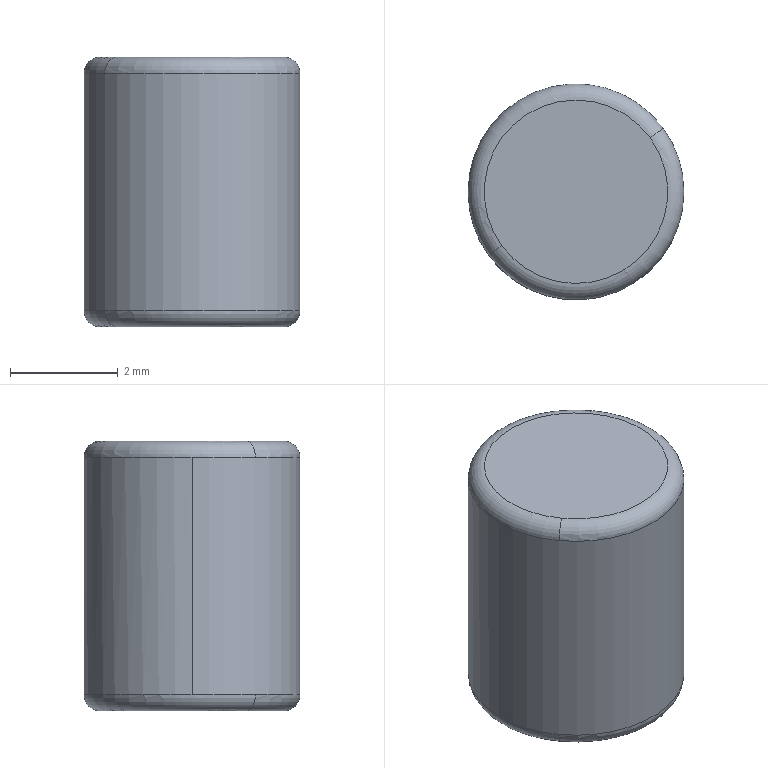Part | 1 solid | 8 faces | box 4 x 4 x 5 mm | volume 62.363 mm3 | torus 4 | cylinder 2 | plane 2 | commonest cylinder face diameters 4 x2
STEP:
#1=CARTESIAN_POINT('',(0.,0.,0.));
#2=DIRECTION('',(0.,0.,1.));
#3=DIRECTION('',(1.,0.,0.));
#4=AXIS2_PLACEMENT_3D('',#1,#2,#3);
#5=CARTESIAN_POINT('',(-242.098,492.5,-190.901));
#6=VERTEX_POINT('',#5);
#7=CARTESIAN_POINT('',(-242.098,492.5,-195.301));
#8=VERTEX_POINT('',#7);
#9=CARTESIAN_POINT('',(-242.098,492.5,-190.901));
#10=DIRECTION('',(0.,0.,-1.));
#11=VECTOR('',#10,1.);
#12=LINE('',#9,#11);
#13=CARTESIAN_POINT('',(-240.098,492.5,-190.601));
#14=DIRECTION('',(0.,0.,-1.));
#15=DIRECTION('',(0.,-1.,0.));
#16=AXIS2_PLACEMENT_3D('',#13,#14,#15);
#17=CYLINDRICAL_SURFACE('',#16,2.);
#18=CARTESIAN_POINT('',(1.571,0.3));
#19=DIRECTION('',(0.,1.));
#20=VECTOR('',#19,1.);
#21=LINE('',#18,#20);
#22=(GEOMETRIC_REPRESENTATION_CONTEXT(2)PARAMETRIC_REPRESENTATION_CONTEXT()REPRESENTATION_CONTEXT('',''));
#23=DEFINITIONAL_REPRESENTATION('',(#21),#22);
#24=PCURVE('',#17,#23);
#25=CARTESIAN_POINT('',(-240.098,492.5,-190.601));
#26=DIRECTION('',(0.,0.,-1.));
#27=DIRECTION('',(0.,1.,0.));
#28=AXIS2_PLACEMENT_3D('',#25,#26,#27);
#29=CYLINDRICAL_SURFACE('',#28,2.);
#30=CARTESIAN_POINT('',(4.712,0.3));
#31=DIRECTION('',(0.,1.));
#32=VECTOR('',#31,1.);
#33=LINE('',#30,#32);
#34=(GEOMETRIC_REPRESENTATION_CONTEXT(2)PARAMETRIC_REPRESENTATION_CONTEXT()REPRESENTATION_CONTEXT('',''));
#35=DEFINITIONAL_REPRESENTATION('',(#33),#34);
#36=PCURVE('',#29,#35);
#37=SURFACE_CURVE('',#12,(#24,#36),.PCURVE_S1.);
#38=EDGE_CURVE('',#6,#8,#37,.T.);
#39=ORIENTED_EDGE('',*,*,#38,.F.);
#40=CARTESIAN_POINT('',(-238.48,493.676,-190.901));
#41=VERTEX_POINT('',#40);
#42=CARTESIAN_POINT('',(-240.098,492.5,-190.901));
#43=DIRECTION('',(0.,0.,-1.));
#44=DIRECTION('',(-1.,0.,0.));
#45=AXIS2_PLACEMENT_3D('',#42,#43,#44);
#46=CIRCLE('',#45,2.);
#47=CARTESIAN_POINT('',(1.571,0.3));
#48=DIRECTION('',(1.,0.));
#49=VECTOR('',#48,1.);
#50=LINE('',#47,#49);
#51=(GEOMETRIC_REPRESENTATION_CONTEXT(2)PARAMETRIC_REPRESENTATION_CONTEXT()REPRESENTATION_CONTEXT('',''));
#52=DEFINITIONAL_REPRESENTATION('',(#50),#51);
#53=PCURVE('',#17,#52);
#54=CARTESIAN_POINT('',(-240.098,492.5,-190.901));
#55=DIRECTION('',(0.,0.,-1.));
#56=DIRECTION('',(0.5878,-0.809,0.));
#57=AXIS2_PLACEMENT_3D('',#54,#55,#56);
#58=TOROIDAL_SURFACE('',#57,1.7,0.3);
#59=CARTESIAN_POINT('',(2.199,6.283));
#60=DIRECTION('',(1.,0.));
#61=VECTOR('',#60,1.);
#62=LINE('',#59,#61);
#63=(GEOMETRIC_REPRESENTATION_CONTEXT(2)PARAMETRIC_REPRESENTATION_CONTEXT()REPRESENTATION_CONTEXT('',''));
#64=DEFINITIONAL_REPRESENTATION('',(#62),#63);
#65=PCURVE('',#58,#64);
#66=SURFACE_CURVE('',#46,(#53,#65),.PCURVE_S1.);
#67=EDGE_CURVE('',#6,#41,#66,.T.);
#68=ORIENTED_EDGE('',*,*,#67,.T.);
#69=CARTESIAN_POINT('',(-238.098,492.5,-190.901));
#70=VERTEX_POINT('',#69);
#71=CARTESIAN_POINT('',(-240.098,492.5,-190.901));
#72=DIRECTION('',(0.,0.,-1.));
#73=DIRECTION('',(-1.,0.,0.));
#74=AXIS2_PLACEMENT_3D('',#71,#72,#73);
#75=CIRCLE('',#74,2.);
#76=CARTESIAN_POINT('',(1.571,0.3));
#77=DIRECTION('',(1.,0.));
#78=VECTOR('',#77,1.);
#79=LINE('',#76,#78);
#80=(GEOMETRIC_REPRESENTATION_CONTEXT(2)PARAMETRIC_REPRESENTATION_CONTEXT()REPRESENTATION_CONTEXT('',''));
#81=DEFINITIONAL_REPRESENTATION('',(#79),#80);
#82=PCURVE('',#17,#81);
#83=CARTESIAN_POINT('',(-240.098,492.5,-190.901));
#84=DIRECTION('',(0.,0.,-1.));
#85=DIRECTION('',(-0.5878,0.809,0.));
#86=AXIS2_PLACEMENT_3D('',#83,#84,#85);
#87=TOROIDAL_SURFACE('',#86,1.7,0.3);
#88=CARTESIAN_POINT('',(-0.9425,6.283));
#89=DIRECTION('',(1.,0.));
#90=VECTOR('',#89,1.);
#91=LINE('',#88,#90);
#92=(GEOMETRIC_REPRESENTATION_CONTEXT(2)PARAMETRIC_REPRESENTATION_CONTEXT()REPRESENTATION_CONTEXT('',''));
#93=DEFINITIONAL_REPRESENTATION('',(#91),#92);
#94=PCURVE('',#87,#93);
#95=SURFACE_CURVE('',#75,(#82,#94),.PCURVE_S1.);
#96=EDGE_CURVE('',#41,#70,#95,.T.);
#97=ORIENTED_EDGE('',*,*,#96,.T.);
#98=CARTESIAN_POINT('',(-238.098,492.5,-195.301));
#99=VERTEX_POINT('',#98);
#100=CARTESIAN_POINT('',(-238.098,492.5,-190.901));
#101=DIRECTION('',(0.,0.,-1.));
#102=VECTOR('',#101,1.);
#103=LINE('',#100,#102);
#104=CARTESIAN_POINT('',(4.712,0.3));
#105=DIRECTION('',(0.,1.));
#106=VECTOR('',#105,1.);
#107=LINE('',#104,#106);
#108=(GEOMETRIC_REPRESENTATION_CONTEXT(2)PARAMETRIC_REPRESENTATION_CONTEXT()REPRESENTATION_CONTEXT('',''));
#109=DEFINITIONAL_REPRESENTATION('',(#107),#108);
#110=PCURVE('',#17,#109);
#111=CARTESIAN_POINT('',(1.571,0.3));
#112=DIRECTION('',(0.,1.));
#113=VECTOR('',#112,1.);
#114=LINE('',#111,#113);
#115=(GEOMETRIC_REPRESENTATION_CONTEXT(2)PARAMETRIC_REPRESENTATION_CONTEXT()REPRESENTATION_CONTEXT('',''));
#116=DEFINITIONAL_REPRESENTATION('',(#114),#115);
#117=PCURVE('',#29,#116);
#118=SURFACE_CURVE('',#103,(#110,#117),.PCURVE_S1.);
#119=EDGE_CURVE('',#70,#99,#118,.T.);
#120=ORIENTED_EDGE('',*,*,#119,.T.);
#121=CARTESIAN_POINT('',(-238.48,493.676,-195.301));
#122=VERTEX_POINT('',#121);
#123=CARTESIAN_POINT('',(-240.098,492.5,-195.301));
#124=DIRECTION('',(0.,0.,1.));
#125=DIRECTION('',(-0.809,0.5878,0.));
#126=AXIS2_PLACEMENT_3D('',#123,#124,#125);
#127=CIRCLE('',#126,2.);
#128=CARTESIAN_POINT('',(8.482,4.7));
#129=DIRECTION('',(-1.,0.));
#130=VECTOR('',#129,1.);
#131=LINE('',#128,#130);
#132=(GEOMETRIC_REPRESENTATION_CONTEXT(2)PARAMETRIC_REPRESENTATION_CONTEXT()REPRESENTATION_CONTEXT('',''));
#133=DEFINITIONAL_REPRESENTATION('',(#131),#132);
#134=PCURVE('',#17,#133);
#135=CARTESIAN_POINT('',(-240.098,492.5,-195.301));
#136=DIRECTION('',(0.,0.,-1.));
#137=DIRECTION('',(-0.5878,0.809,0.));
#138=AXIS2_PLACEMENT_3D('',#135,#136,#137);
#139=TOROIDAL_SURFACE('',#138,1.7,0.3);
#140=CARTESIAN_POINT('',(5.969,0.));
#141=DIRECTION('',(-1.,0.));
#142=VECTOR('',#141,1.);
#143=LINE('',#140,#142);
#144=(GEOMETRIC_REPRESENTATION_CONTEXT(2)PARAMETRIC_REPRESENTATION_CONTEXT()REPRESENTATION_CONTEXT('',''));
#145=DEFINITIONAL_REPRESENTATION('',(#143),#144);
#146=PCURVE('',#139,#145);
#147=SURFACE_CURVE('',#127,(#134,#146),.PCURVE_S1.);
#148=EDGE_CURVE('',#99,#122,#147,.T.);
#149=ORIENTED_EDGE('',*,*,#148,.T.);
#150=CARTESIAN_POINT('',(-241.716,493.676,-195.301));
#151=VERTEX_POINT('',#150);
#152=CARTESIAN_POINT('',(-240.098,492.5,-195.301));
#153=DIRECTION('',(0.,0.,1.));
#154=DIRECTION('',(-0.809,0.5878,0.));
#155=AXIS2_PLACEMENT_3D('',#152,#153,#154);
#156=CIRCLE('',#155,2.);
#157=CARTESIAN_POINT('',(8.482,4.7));
#158=DIRECTION('',(-1.,0.));
#159=VECTOR('',#158,1.);
#160=LINE('',#157,#159);
#161=(GEOMETRIC_REPRESENTATION_CONTEXT(2)PARAMETRIC_REPRESENTATION_CONTEXT()REPRESENTATION_CONTEXT('',''));
#162=DEFINITIONAL_REPRESENTATION('',(#160),#161);
#163=PCURVE('',#17,#162);
#164=CARTESIAN_POINT('',(-240.098,492.5,-195.301));
#165=DIRECTION('',(0.,0.,-1.));
#166=DIRECTION('',(0.5878,-0.809,0.));
#167=AXIS2_PLACEMENT_3D('',#164,#165,#166);
#168=TOROIDAL_SURFACE('',#167,1.7,0.3);
#169=CARTESIAN_POINT('',(9.111,0.));
#170=DIRECTION('',(-1.,0.));
#171=VECTOR('',#170,1.);
#172=LINE('',#169,#171);
#173=(GEOMETRIC_REPRESENTATION_CONTEXT(2)PARAMETRIC_REPRESENTATION_CONTEXT()REPRESENTATION_CONTEXT('',''));
#174=DEFINITIONAL_REPRESENTATION('',(#172),#173);
#175=PCURVE('',#168,#174);
#176=SURFACE_CURVE('',#156,(#163,#175),.PCURVE_S1.);
#177=EDGE_CURVE('',#122,#151,#176,.T.);
#178=ORIENTED_EDGE('',*,*,#177,.T.);
#179=CARTESIAN_POINT('',(-240.098,492.5,-195.301));
#180=DIRECTION('',(0.,0.,1.));
#181=DIRECTION('',(-0.809,0.5878,0.));
#182=AXIS2_PLACEMENT_3D('',#179,#180,#181);
#183=CIRCLE('',#182,2.);
#184=CARTESIAN_POINT('',(2.199,4.7));
#185=DIRECTION('',(-1.,0.));
#186=VECTOR('',#185,1.);
#187=LINE('',#184,#186);
#188=(GEOMETRIC_REPRESENTATION_CONTEXT(2)PARAMETRIC_REPRESENTATION_CONTEXT()REPRESENTATION_CONTEXT('',''));
#189=DEFINITIONAL_REPRESENTATION('',(#187),#188);
#190=PCURVE('',#17,#189);
#191=CARTESIAN_POINT('',(2.827,0.));
#192=DIRECTION('',(-1.,0.));
#193=VECTOR('',#192,1.);
#194=LINE('',#191,#193);
#195=(GEOMETRIC_REPRESENTATION_CONTEXT(2)PARAMETRIC_REPRESENTATION_CONTEXT()REPRESENTATION_CONTEXT('',''));
#196=DEFINITIONAL_REPRESENTATION('',(#194),#195);
#197=PCURVE('',#168,#196);
#198=SURFACE_CURVE('',#183,(#190,#197),.PCURVE_S1.);
#199=EDGE_CURVE('',#151,#8,#198,.T.);
#200=ORIENTED_EDGE('',*,*,#199,.T.);
#201=EDGE_LOOP('',(#39,#68,#97,#120,#149,#178,#200));
#202=FACE_BOUND('',#201,.T.);
#203=ADVANCED_FACE('',(#202),#17,.T.);
#204=CARTESIAN_POINT('',(-241.474,491.501,-195.601));
#205=VERTEX_POINT('',#204);
#206=CARTESIAN_POINT('',(-241.716,491.325,-195.301));
#207=VERTEX_POINT('',#206);
#208=CARTESIAN_POINT('',(-241.474,491.501,-195.301));
#209=DIRECTION('',(-0.5878,0.809,0.));
#210=DIRECTION('',(0.,0.,-1.));
#211=AXIS2_PLACEMENT_3D('',#208,#209,#210);
#212=CIRCLE('',#211,0.3);
#213=CARTESIAN_POINT('',(1.571,1.571));
#214=DIRECTION('',(0.,-1.));
#215=VECTOR('',#214,1.);
#216=LINE('',#213,#215);
#217=(GEOMETRIC_REPRESENTATION_CONTEXT(2)PARAMETRIC_REPRESENTATION_CONTEXT()REPRESENTATION_CONTEXT('',''));
#218=DEFINITIONAL_REPRESENTATION('',(#216),#217);
#219=PCURVE('',#168,#218);
#220=CARTESIAN_POINT('',(4.712,1.571));
#221=DIRECTION('',(0.,-1.));
#222=VECTOR('',#221,1.);
#223=LINE('',#220,#222);
#224=(GEOMETRIC_REPRESENTATION_CONTEXT(2)PARAMETRIC_REPRESENTATION_CONTEXT()REPRESENTATION_CONTEXT('',''));
#225=DEFINITIONAL_REPRESENTATION('',(#223),#224);
#226=PCURVE('',#139,#225);
#227=SURFACE_CURVE('',#212,(#219,#226),.PCURVE_S1.);
#228=EDGE_CURVE('',#205,#207,#227,.T.);
#229=ORIENTED_EDGE('',*,*,#228,.T.);
#230=CARTESIAN_POINT('',(-240.098,492.5,-195.301));
#231=DIRECTION('',(0.,0.,1.));
#232=DIRECTION('',(-0.809,0.5878,0.));
#233=AXIS2_PLACEMENT_3D('',#230,#231,#232);
#234=CIRCLE('',#233,2.);
#235=CARTESIAN_POINT('',(2.827,0.));
#236=DIRECTION('',(-1.,0.));
#237=VECTOR('',#236,1.);
#238=LINE('',#235,#237);
#239=(GEOMETRIC_REPRESENTATION_CONTEXT(2)PARAMETRIC_REPRESENTATION_CONTEXT()REPRESENTATION_CONTEXT('',''));
#240=DEFINITIONAL_REPRESENTATION('',(#238),#239);
#241=PCURVE('',#168,#240);
#242=CARTESIAN_POINT('',(5.341,4.7));
#243=DIRECTION('',(-1.,0.));
#244=VECTOR('',#243,1.);
#245=LINE('',#242,#244);
#246=(GEOMETRIC_REPRESENTATION_CONTEXT(2)PARAMETRIC_REPRESENTATION_CONTEXT()REPRESENTATION_CONTEXT('',''));
#247=DEFINITIONAL_REPRESENTATION('',(#245),#246);
#248=PCURVE('',#29,#247);
#249=SURFACE_CURVE('',#234,(#241,#248),.PCURVE_S1.);
#250=EDGE_CURVE('',#8,#207,#249,.T.);
#251=ORIENTED_EDGE('',*,*,#250,.F.);
#252=ORIENTED_EDGE('',*,*,#199,.F.);
#253=ORIENTED_EDGE('',*,*,#177,.F.);
#254=CARTESIAN_POINT('',(-238.723,493.5,-195.601));
#255=VERTEX_POINT('',#254);
#256=CARTESIAN_POINT('',(-238.723,493.5,-195.301));
#257=DIRECTION('',(0.5878,-0.809,0.));
#258=DIRECTION('',(0.,0.,-1.));
#259=AXIS2_PLACEMENT_3D('',#256,#257,#258);
#260=CIRCLE('',#259,0.3);
#261=CARTESIAN_POINT('',(4.712,1.571));
#262=DIRECTION('',(0.,-1.));
#263=VECTOR('',#262,1.);
#264=LINE('',#261,#263);
#265=(GEOMETRIC_REPRESENTATION_CONTEXT(2)PARAMETRIC_REPRESENTATION_CONTEXT()REPRESENTATION_CONTEXT('',''));
#266=DEFINITIONAL_REPRESENTATION('',(#264),#265);
#267=PCURVE('',#168,#266);
#268=CARTESIAN_POINT('',(1.571,1.571));
#269=DIRECTION('',(0.,-1.));
#270=VECTOR('',#269,1.);
#271=LINE('',#268,#270);
#272=(GEOMETRIC_REPRESENTATION_CONTEXT(2)PARAMETRIC_REPRESENTATION_CONTEXT()REPRESENTATION_CONTEXT('',''));
#273=DEFINITIONAL_REPRESENTATION('',(#271),#272);
#274=PCURVE('',#139,#273);
#275=SURFACE_CURVE('',#260,(#267,#274),.PCURVE_S1.);
#276=EDGE_CURVE('',#255,#122,#275,.T.);
#277=ORIENTED_EDGE('',*,*,#276,.F.);
#278=CARTESIAN_POINT('',(-241.474,493.5,-195.601));
#279=VERTEX_POINT('',#278);
#280=CARTESIAN_POINT('',(-240.098,492.5,-195.601));
#281=DIRECTION('',(0.,0.,-1.));
#282=DIRECTION('',(-0.809,0.5878,0.));
#283=AXIS2_PLACEMENT_3D('',#280,#281,#282);
#284=CIRCLE('',#283,1.7);
#285=CARTESIAN_POINT('',(2.827,1.571));
#286=DIRECTION('',(1.,0.));
#287=VECTOR('',#286,1.);
#288=LINE('',#285,#287);
#289=(GEOMETRIC_REPRESENTATION_CONTEXT(2)PARAMETRIC_REPRESENTATION_CONTEXT()REPRESENTATION_CONTEXT('',''));
#290=DEFINITIONAL_REPRESENTATION('',(#288),#289);
#291=PCURVE('',#168,#290);
#292=CARTESIAN_POINT('',(-240.098,492.5,-195.601));
#293=DIRECTION('',(0.,0.,-1.));
#294=DIRECTION('',(1.,0.,0.));
#295=AXIS2_PLACEMENT_3D('',#292,#293,#294);
#296=PLANE('',#295);
#297=CARTESIAN_POINT('',(0.,0.));
#298=DIRECTION('',(-0.809,-0.5878));
#299=AXIS2_PLACEMENT_2D('',#297,#298);
#300=CIRCLE('',#299,1.7);
#301=(GEOMETRIC_REPRESENTATION_CONTEXT(2)PARAMETRIC_REPRESENTATION_CONTEXT()REPRESENTATION_CONTEXT('',''));
#302=DEFINITIONAL_REPRESENTATION('',(#300),#301);
#303=PCURVE('',#296,#302);
#304=SURFACE_CURVE('',#284,(#291,#303),.PCURVE_S1.);
#305=EDGE_CURVE('',#279,#255,#304,.T.);
#306=ORIENTED_EDGE('',*,*,#305,.F.);
#307=CARTESIAN_POINT('',(-240.098,492.5,-195.601));
#308=DIRECTION('',(0.,0.,-1.));
#309=DIRECTION('',(-0.809,0.5878,0.));
#310=AXIS2_PLACEMENT_3D('',#307,#308,#309);
#311=CIRCLE('',#310,1.7);
#312=CARTESIAN_POINT('',(-3.456,1.571));
#313=DIRECTION('',(1.,0.));
#314=VECTOR('',#313,1.);
#315=LINE('',#312,#314);
#316=(GEOMETRIC_REPRESENTATION_CONTEXT(2)PARAMETRIC_REPRESENTATION_CONTEXT()REPRESENTATION_CONTEXT('',''));
#317=DEFINITIONAL_REPRESENTATION('',(#315),#316);
#318=PCURVE('',#168,#317);
#319=CARTESIAN_POINT('',(0.,0.));
#320=DIRECTION('',(-0.809,-0.5878));
#321=AXIS2_PLACEMENT_2D('',#319,#320);
#322=CIRCLE('',#321,1.7);
#323=(GEOMETRIC_REPRESENTATION_CONTEXT(2)PARAMETRIC_REPRESENTATION_CONTEXT()REPRESENTATION_CONTEXT('',''));
#324=DEFINITIONAL_REPRESENTATION('',(#322),#323);
#325=PCURVE('',#296,#324);
#326=SURFACE_CURVE('',#311,(#318,#325),.PCURVE_S1.);
#327=EDGE_CURVE('',#205,#279,#326,.T.);
#328=ORIENTED_EDGE('',*,*,#327,.F.);
#329=EDGE_LOOP('',(#229,#251,#252,#253,#277,#306,#328));
#330=FACE_BOUND('',#329,.T.);
#331=ADVANCED_FACE('',(#330),#168,.T.);
#332=ORIENTED_EDGE('',*,*,#305,.T.);
#333=CARTESIAN_POINT('',(-240.098,492.5,-195.601));
#334=DIRECTION('',(0.,0.,-1.));
#335=DIRECTION('',(-0.809,0.5878,0.));
#336=AXIS2_PLACEMENT_3D('',#333,#334,#335);
#337=CIRCLE('',#336,1.7);
#338=CARTESIAN_POINT('',(0.,0.));
#339=DIRECTION('',(-0.809,-0.5878));
#340=AXIS2_PLACEMENT_2D('',#338,#339);
#341=CIRCLE('',#340,1.7);
#342=(GEOMETRIC_REPRESENTATION_CONTEXT(2)PARAMETRIC_REPRESENTATION_CONTEXT()REPRESENTATION_CONTEXT('',''));
#343=DEFINITIONAL_REPRESENTATION('',(#341),#342);
#344=PCURVE('',#296,#343);
#345=CARTESIAN_POINT('',(-0.3142,1.571));
#346=DIRECTION('',(1.,0.));
#347=VECTOR('',#346,1.);
#348=LINE('',#345,#347);
#349=(GEOMETRIC_REPRESENTATION_CONTEXT(2)PARAMETRIC_REPRESENTATION_CONTEXT()REPRESENTATION_CONTEXT('',''));
#350=DEFINITIONAL_REPRESENTATION('',(#348),#349);
#351=PCURVE('',#139,#350);
#352=SURFACE_CURVE('',#337,(#344,#351),.PCURVE_S1.);
#353=EDGE_CURVE('',#255,#205,#352,.T.);
#354=ORIENTED_EDGE('',*,*,#353,.T.);
#355=ORIENTED_EDGE('',*,*,#327,.T.);
#356=EDGE_LOOP('',(#332,#354,#355));
#357=FACE_BOUND('',#356,.T.);
#358=ADVANCED_FACE('',(#357),#296,.T.);
#359=CARTESIAN_POINT('',(-241.716,491.325,-190.901));
#360=VERTEX_POINT('',#359);
#361=CARTESIAN_POINT('',(-241.474,491.501,-190.601));
#362=VERTEX_POINT('',#361);
#363=CARTESIAN_POINT('',(-241.474,491.501,-190.901));
#364=DIRECTION('',(-0.5878,0.809,0.));
#365=DIRECTION('',(-0.809,-0.5878,0.));
#366=AXIS2_PLACEMENT_3D('',#363,#364,#365);
#367=CIRCLE('',#366,0.3);
#368=CARTESIAN_POINT('',(1.571,6.283));
#369=DIRECTION('',(0.,-1.));
#370=VECTOR('',#369,1.);
#371=LINE('',#368,#370);
#372=(GEOMETRIC_REPRESENTATION_CONTEXT(2)PARAMETRIC_REPRESENTATION_CONTEXT()REPRESENTATION_CONTEXT('',''));
#373=DEFINITIONAL_REPRESENTATION('',(#371),#372);
#374=PCURVE('',#58,#373);
#375=CARTESIAN_POINT('',(4.712,6.283));
#376=DIRECTION('',(0.,-1.));
#377=VECTOR('',#376,1.);
#378=LINE('',#375,#377);
#379=(GEOMETRIC_REPRESENTATION_CONTEXT(2)PARAMETRIC_REPRESENTATION_CONTEXT()REPRESENTATION_CONTEXT('',''));
#380=DEFINITIONAL_REPRESENTATION('',(#378),#379);
#381=PCURVE('',#87,#380);
#382=SURFACE_CURVE('',#367,(#374,#381),.PCURVE_S1.);
#383=EDGE_CURVE('',#360,#362,#382,.T.);
#384=ORIENTED_EDGE('',*,*,#383,.T.);
#385=CARTESIAN_POINT('',(-241.474,493.5,-190.601));
#386=VERTEX_POINT('',#385);
#387=CARTESIAN_POINT('',(-240.098,492.5,-190.601));
#388=DIRECTION('',(0.,0.,1.));
#389=DIRECTION('',(-0.809,0.5878,0.));
#390=AXIS2_PLACEMENT_3D('',#387,#388,#389);
#391=CIRCLE('',#390,1.7);
#392=CARTESIAN_POINT('',(2.827,4.712));
#393=DIRECTION('',(-1.,0.));
#394=VECTOR('',#393,1.);
#395=LINE('',#392,#394);
#396=(GEOMETRIC_REPRESENTATION_CONTEXT(2)PARAMETRIC_REPRESENTATION_CONTEXT()REPRESENTATION_CONTEXT('',''));
#397=DEFINITIONAL_REPRESENTATION('',(#395),#396);
#398=PCURVE('',#58,#397);
#399=CARTESIAN_POINT('',(-240.098,492.5,-190.601));
#400=DIRECTION('',(0.,0.,-1.));
#401=DIRECTION('',(1.,0.,0.));
#402=AXIS2_PLACEMENT_3D('',#399,#400,#401);
#403=PLANE('',#402);
#404=CARTESIAN_POINT('',(-1.375,-0.9992));
#405=CARTESIAN_POINT('',(-3.106,1.383));
#406=CARTESIAN_POINT('',(-0.1777,1.691));
#407=CARTESIAN_POINT('',(2.751,1.998));
#408=CARTESIAN_POINT('',(1.553,-0.6915));
#409=CARTESIAN_POINT('',(0.3554,-3.381));
#410=CARTESIAN_POINT('',(-1.375,-0.9992));
#411=(BOUNDED_CURVE()B_SPLINE_CURVE(2,(#404,#405,#406,#407,#408,#409,#410),.UNSPECIFIED.,.T.,.F.)B_SPLINE_CURVE_WITH_KNOTS((1,2,2,2,2,1),(-2.094,0.,2.094,4.189,6.283,8.378),.UNSPECIFIED.)CURVE()GEOMETRIC_REPRESENTATION_ITEM()RATIONAL_B_SPLINE_CURVE((1.,0.5,1.,0.5,1.,0.5,1.))REPRESENTATION_ITEM(''));
#412=(GEOMETRIC_REPRESENTATION_CONTEXT(2)PARAMETRIC_REPRESENTATION_CONTEXT()REPRESENTATION_CONTEXT('',''));
#413=DEFINITIONAL_REPRESENTATION('',(#411),#412);
#414=PCURVE('',#403,#413);
#415=SURFACE_CURVE('',#391,(#398,#414),.PCURVE_S1.);
#416=EDGE_CURVE('',#386,#362,#415,.T.);
#417=ORIENTED_EDGE('',*,*,#416,.F.);
#418=CARTESIAN_POINT('',(-238.723,493.5,-190.601));
#419=VERTEX_POINT('',#418);
#420=CARTESIAN_POINT('',(-240.098,492.5,-190.601));
#421=DIRECTION('',(0.,0.,1.));
#422=DIRECTION('',(-0.809,0.5878,0.));
#423=AXIS2_PLACEMENT_3D('',#420,#421,#422);
#424=CIRCLE('',#423,1.7);
#425=CARTESIAN_POINT('',(9.111,4.712));
#426=DIRECTION('',(-1.,0.));
#427=VECTOR('',#426,1.);
#428=LINE('',#425,#427);
#429=(GEOMETRIC_REPRESENTATION_CONTEXT(2)PARAMETRIC_REPRESENTATION_CONTEXT()REPRESENTATION_CONTEXT('',''));
#430=DEFINITIONAL_REPRESENTATION('',(#428),#429);
#431=PCURVE('',#58,#430);
#432=CARTESIAN_POINT('',(-1.375,-0.9992));
#433=CARTESIAN_POINT('',(-3.106,1.383));
#434=CARTESIAN_POINT('',(-0.1777,1.691));
#435=CARTESIAN_POINT('',(2.751,1.998));
#436=CARTESIAN_POINT('',(1.553,-0.6915));
#437=CARTESIAN_POINT('',(0.3554,-3.381));
#438=CARTESIAN_POINT('',(-1.375,-0.9992));
#439=(BOUNDED_CURVE()B_SPLINE_CURVE(2,(#432,#433,#434,#435,#436,#437,#438),.UNSPECIFIED.,.T.,.F.)B_SPLINE_CURVE_WITH_KNOTS((1,2,2,2,2,1),(-2.094,0.,2.094,4.189,6.283,8.378),.UNSPECIFIED.)CURVE()GEOMETRIC_REPRESENTATION_ITEM()RATIONAL_B_SPLINE_CURVE((1.,0.5,1.,0.5,1.,0.5,1.))REPRESENTATION_ITEM(''));
#440=(GEOMETRIC_REPRESENTATION_CONTEXT(2)PARAMETRIC_REPRESENTATION_CONTEXT()REPRESENTATION_CONTEXT('',''));
#441=DEFINITIONAL_REPRESENTATION('',(#439),#440);
#442=PCURVE('',#403,#441);
#443=SURFACE_CURVE('',#424,(#431,#442),.PCURVE_S1.);
#444=EDGE_CURVE('',#419,#386,#443,.T.);
#445=ORIENTED_EDGE('',*,*,#444,.F.);
#446=CARTESIAN_POINT('',(-238.723,493.5,-190.901));
#447=DIRECTION('',(0.5878,-0.809,0.));
#448=DIRECTION('',(0.809,0.5878,0.));
#449=AXIS2_PLACEMENT_3D('',#446,#447,#448);
#450=CIRCLE('',#449,0.3);
#451=CARTESIAN_POINT('',(4.712,6.283));
#452=DIRECTION('',(0.,-1.));
#453=VECTOR('',#452,1.);
#454=LINE('',#451,#453);
#455=(GEOMETRIC_REPRESENTATION_CONTEXT(2)PARAMETRIC_REPRESENTATION_CONTEXT()REPRESENTATION_CONTEXT('',''));
#456=DEFINITIONAL_REPRESENTATION('',(#454),#455);
#457=PCURVE('',#58,#456);
#458=CARTESIAN_POINT('',(1.571,6.283));
#459=DIRECTION('',(0.,-1.));
#460=VECTOR('',#459,1.);
#461=LINE('',#458,#460);
#462=(GEOMETRIC_REPRESENTATION_CONTEXT(2)PARAMETRIC_REPRESENTATION_CONTEXT()REPRESENTATION_CONTEXT('',''));
#463=DEFINITIONAL_REPRESENTATION('',(#461),#462);
#464=PCURVE('',#87,#463);
#465=SURFACE_CURVE('',#450,(#457,#464),.PCURVE_S1.);
#466=EDGE_CURVE('',#41,#419,#465,.T.);
#467=ORIENTED_EDGE('',*,*,#466,.F.);
#468=ORIENTED_EDGE('',*,*,#67,.F.);
#469=CARTESIAN_POINT('',(-240.098,492.5,-190.901));
#470=DIRECTION('',(0.,0.,-1.));
#471=DIRECTION('',(-1.,0.,0.));
#472=AXIS2_PLACEMENT_3D('',#469,#470,#471);
#473=CIRCLE('',#472,2.);
#474=CARTESIAN_POINT('',(-4.084,6.283));
#475=DIRECTION('',(1.,0.));
#476=VECTOR('',#475,1.);
#477=LINE('',#474,#476);
#478=(GEOMETRIC_REPRESENTATION_CONTEXT(2)PARAMETRIC_REPRESENTATION_CONTEXT()REPRESENTATION_CONTEXT('',''));
#479=DEFINITIONAL_REPRESENTATION('',(#477),#478);
#480=PCURVE('',#58,#479);
#481=CARTESIAN_POINT('',(-1.571,0.3));
#482=DIRECTION('',(1.,0.));
#483=VECTOR('',#482,1.);
#484=LINE('',#481,#483);
#485=(GEOMETRIC_REPRESENTATION_CONTEXT(2)PARAMETRIC_REPRESENTATION_CONTEXT()REPRESENTATION_CONTEXT('',''));
#486=DEFINITIONAL_REPRESENTATION('',(#484),#485);
#487=PCURVE('',#29,#486);
#488=SURFACE_CURVE('',#473,(#480,#487),.PCURVE_S1.);
#489=EDGE_CURVE('',#360,#6,#488,.T.);
#490=ORIENTED_EDGE('',*,*,#489,.F.);
#491=EDGE_LOOP('',(#384,#417,#445,#467,#468,#490));
#492=FACE_BOUND('',#491,.T.);
#493=ADVANCED_FACE('',(#492),#58,.T.);
#494=ORIENTED_EDGE('',*,*,#416,.T.);
#495=CARTESIAN_POINT('',(-240.098,492.5,-190.601));
#496=DIRECTION('',(0.,0.,1.));
#497=DIRECTION('',(-0.809,0.5878,0.));
#498=AXIS2_PLACEMENT_3D('',#495,#496,#497);
#499=CIRCLE('',#498,1.7);
#500=CARTESIAN_POINT('',(-1.375,-0.9992));
#501=CARTESIAN_POINT('',(-3.106,1.383));
#502=CARTESIAN_POINT('',(-0.1777,1.691));
#503=CARTESIAN_POINT('',(2.751,1.998));
#504=CARTESIAN_POINT('',(1.553,-0.6915));
#505=CARTESIAN_POINT('',(0.3554,-3.381));
#506=CARTESIAN_POINT('',(-1.375,-0.9992));
#507=(BOUNDED_CURVE()B_SPLINE_CURVE(2,(#500,#501,#502,#503,#504,#505,#506),.UNSPECIFIED.,.T.,.F.)B_SPLINE_CURVE_WITH_KNOTS((1,2,2,2,2,1),(-2.094,0.,2.094,4.189,6.283,8.378),.UNSPECIFIED.)CURVE()GEOMETRIC_REPRESENTATION_ITEM()RATIONAL_B_SPLINE_CURVE((1.,0.5,1.,0.5,1.,0.5,1.))REPRESENTATION_ITEM(''));
#508=(GEOMETRIC_REPRESENTATION_CONTEXT(2)PARAMETRIC_REPRESENTATION_CONTEXT()REPRESENTATION_CONTEXT('',''));
#509=DEFINITIONAL_REPRESENTATION('',(#507),#508);
#510=PCURVE('',#403,#509);
#511=CARTESIAN_POINT('',(5.969,4.712));
#512=DIRECTION('',(-1.,0.));
#513=VECTOR('',#512,1.);
#514=LINE('',#511,#513);
#515=(GEOMETRIC_REPRESENTATION_CONTEXT(2)PARAMETRIC_REPRESENTATION_CONTEXT()REPRESENTATION_CONTEXT('',''));
#516=DEFINITIONAL_REPRESENTATION('',(#514),#515);
#517=PCURVE('',#87,#516);
#518=SURFACE_CURVE('',#499,(#510,#517),.PCURVE_S1.);
#519=EDGE_CURVE('',#362,#419,#518,.T.);
#520=ORIENTED_EDGE('',*,*,#519,.T.);
#521=ORIENTED_EDGE('',*,*,#444,.T.);
#522=EDGE_LOOP('',(#494,#520,#521));
#523=FACE_BOUND('',#522,.T.);
#524=ADVANCED_FACE('',(#523),#403,.F.);
#525=ORIENTED_EDGE('',*,*,#38,.T.);
#526=ORIENTED_EDGE('',*,*,#250,.T.);
#527=CARTESIAN_POINT('',(-240.098,492.5,-195.301));
#528=DIRECTION('',(0.,0.,1.));
#529=DIRECTION('',(-0.809,0.5878,0.));
#530=AXIS2_PLACEMENT_3D('',#527,#528,#529);
#531=CIRCLE('',#530,2.);
#532=CARTESIAN_POINT('',(5.341,4.7));
#533=DIRECTION('',(-1.,0.));
#534=VECTOR('',#533,1.);
#535=LINE('',#532,#534);
#536=(GEOMETRIC_REPRESENTATION_CONTEXT(2)PARAMETRIC_REPRESENTATION_CONTEXT()REPRESENTATION_CONTEXT('',''));
#537=DEFINITIONAL_REPRESENTATION('',(#535),#536);
#538=PCURVE('',#29,#537);
#539=CARTESIAN_POINT('',(5.969,0.));
#540=DIRECTION('',(-1.,0.));
#541=VECTOR('',#540,1.);
#542=LINE('',#539,#541);
#543=(GEOMETRIC_REPRESENTATION_CONTEXT(2)PARAMETRIC_REPRESENTATION_CONTEXT()REPRESENTATION_CONTEXT('',''));
#544=DEFINITIONAL_REPRESENTATION('',(#542),#543);
#545=PCURVE('',#139,#544);
#546=SURFACE_CURVE('',#531,(#538,#545),.PCURVE_S1.);
#547=EDGE_CURVE('',#207,#99,#546,.T.);
#548=ORIENTED_EDGE('',*,*,#547,.T.);
#549=ORIENTED_EDGE('',*,*,#119,.F.);
#550=CARTESIAN_POINT('',(-240.098,492.5,-190.901));
#551=DIRECTION('',(0.,0.,-1.));
#552=DIRECTION('',(-1.,0.,0.));
#553=AXIS2_PLACEMENT_3D('',#550,#551,#552);
#554=CIRCLE('',#553,2.);
#555=CARTESIAN_POINT('',(-1.571,0.3));
#556=DIRECTION('',(1.,0.));
#557=VECTOR('',#556,1.);
#558=LINE('',#555,#557);
#559=(GEOMETRIC_REPRESENTATION_CONTEXT(2)PARAMETRIC_REPRESENTATION_CONTEXT()REPRESENTATION_CONTEXT('',''));
#560=DEFINITIONAL_REPRESENTATION('',(#558),#559);
#561=PCURVE('',#29,#560);
#562=CARTESIAN_POINT('',(-0.9425,6.283));
#563=DIRECTION('',(1.,0.));
#564=VECTOR('',#563,1.);
#565=LINE('',#562,#564);
#566=(GEOMETRIC_REPRESENTATION_CONTEXT(2)PARAMETRIC_REPRESENTATION_CONTEXT()REPRESENTATION_CONTEXT('',''));
#567=DEFINITIONAL_REPRESENTATION('',(#565),#566);
#568=PCURVE('',#87,#567);
#569=SURFACE_CURVE('',#554,(#561,#568),.PCURVE_S1.);
#570=EDGE_CURVE('',#70,#360,#569,.T.);
#571=ORIENTED_EDGE('',*,*,#570,.T.);
#572=ORIENTED_EDGE('',*,*,#489,.T.);
#573=EDGE_LOOP('',(#525,#526,#548,#549,#571,#572));
#574=FACE_BOUND('',#573,.T.);
#575=ADVANCED_FACE('',(#574),#29,.T.);
#576=ORIENTED_EDGE('',*,*,#228,.F.);
#577=ORIENTED_EDGE('',*,*,#353,.F.);
#578=ORIENTED_EDGE('',*,*,#276,.T.);
#579=ORIENTED_EDGE('',*,*,#148,.F.);
#580=ORIENTED_EDGE('',*,*,#547,.F.);
#581=EDGE_LOOP('',(#576,#577,#578,#579,#580));
#582=FACE_BOUND('',#581,.T.);
#583=ADVANCED_FACE('',(#582),#139,.T.);
#584=ORIENTED_EDGE('',*,*,#383,.F.);
#585=ORIENTED_EDGE('',*,*,#570,.F.);
#586=ORIENTED_EDGE('',*,*,#96,.F.);
#587=ORIENTED_EDGE('',*,*,#466,.T.);
#588=ORIENTED_EDGE('',*,*,#519,.F.);
#589=EDGE_LOOP('',(#584,#585,#586,#587,#588));
#590=FACE_BOUND('',#589,.T.);
#591=ADVANCED_FACE('',(#590),#87,.T.);
#592=CLOSED_SHELL('',(#203,#331,#358,#493,#524,#575,#583,#591));
#593=MANIFOLD_SOLID_BREP('',#592);
#594=(LENGTH_UNIT()NAMED_UNIT(*)SI_UNIT(.MILLI.,.METRE.));
#595=UNCERTAINTY_MEASURE_WITH_UNIT(LENGTH_MEASURE(0.0000001),#594,'','');
#596=(NAMED_UNIT(*)PLANE_ANGLE_UNIT()SI_UNIT($,.RADIAN.));
#597=(NAMED_UNIT(*)SI_UNIT($,.STERADIAN.)SOLID_ANGLE_UNIT());
#598=(GEOMETRIC_REPRESENTATION_CONTEXT(3)GLOBAL_UNCERTAINTY_ASSIGNED_CONTEXT((#595))GLOBAL_UNIT_ASSIGNED_CONTEXT((#594,#596,#597))REPRESENTATION_CONTEXT('',''));
#599=ADVANCED_BREP_SHAPE_REPRESENTATION('',(#4,#593),#598);